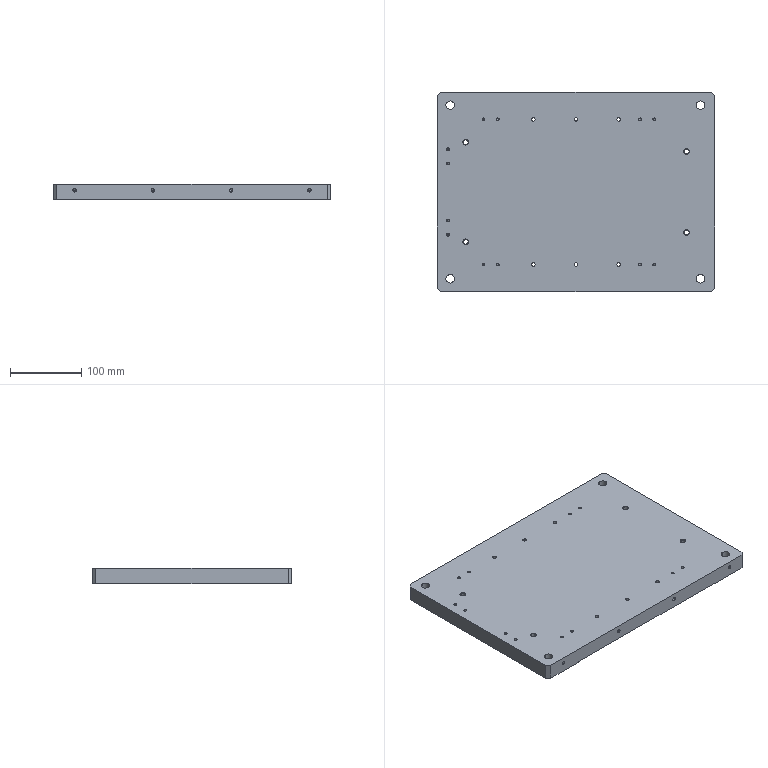NC program | NX | posted with a generic post | part box 390 x 280 x 22 mm
Whole program:
N10 G17 G21 G94 G90
(FLOOR_WALL_COPY , TOOL : D20R0.8)
N12 T01 M6
N14 G54
N16 G17 G0 G90 X208. Y-139.999 S7500 M3
N18 G43 Z30. H1
N20 Z3.
N22 G94 G1 Z0. F1350.
N24 X205.
N26 X-205.
N28 Y-130.262
N30 X205.
N32 Y-120.525
N34 X-205.
N36 Y-115.134
N38 Y-110.788
N40 X205.
N42 Y-101.051
N44 X-205.
N46 Y-91.313
N48 X205.
N50 Y-81.576
N52 X-205.
N54 Y-71.839
N56 X205.
N58 Y-62.102
N60 X-205.
N62 Y-52.365
N64 X205.
N66 Y-42.628
N68 X-205.
N70 Y-32.891
N72 X205.
N74 Y-23.154
N76 X-205.
N78 Y-13.417
N80 X205.
N82 Y-3.68
N84 X-205.
N86 Y6.058
N88 X205.
N90 Y15.795
N92 X-205.
N94 Y25.532
N96 X205.
N98 Y35.269
N100 X-205.
N102 Y45.006
N104 X205.
N106 Y54.743
N108 X-205.
N110 Y64.48
N112 X205.
N114 Y74.217
N116 X-205.
N118 Y83.954
N120 X205.
N122 Y93.692
N124 X-205.
N126 Y103.429
N128 X205.
N130 Y113.166
N132 X-205.
N134 Y122.903
N136 X205.
N138 Y132.64
N140 X-205.
N142 X-208.
N144 Z3.
N146 G0 Z30.
N148 M5
(FLOOR_WALL_1 , TOOL : D10)
N150 T02 M6
N152 G54
N154 G17 G0 G90 X129.897 Y148.1 S9500 M3
N156 G43 Z30. H2
N158 Z2.7
N160 G94 G1 Z-0.3 F2500.
N162 Y145.
N164 Y-145.
N166 X122.474
N168 Y145.
N170 X115.051
N172 Y-145.
N174 X107.629
N176 Y145.
N178 X100.206
N180 Y-145.
N182 X92.783
N184 Y145.
N186 X85.36
N188 Y-145.
N190 X77.938
N192 Y145.
N194 X70.515
N196 Y-145.
N198 X63.092
N200 Y145.
N202 X55.669
N204 Y-145.
N206 X48.247
N208 Y145.
N210 X40.824
N212 Y-145.
N214 X33.401
N216 Y145.
N218 X25.978
N220 Y-145.
N222 X18.555
N224 Y145.
N226 X11.133
N228 Y-145.
N230 X3.71
N232 Y145.
N234 X-3.713
N236 Y-145.
N238 X-11.136
N240 Y145.
N242 X-18.558
N244 Y-145.
N246 X-25.981
N248 Y145.
N250 X-33.404
N252 Y-145.
N254 X-40.827
N256 Y145.
N258 X-48.25
N260 Y-145.
N262 X-55.672
N264 Y145.
N266 X-63.095
N268 Y-145.
N270 X-70.518
N272 Y145.
N274 X-77.941
N276 Y-145.
N278 X-85.363
N280 Y145.
N282 X-92.786
N284 Y-145.
N286 X-100.209
N288 Y145.
N290 X-107.632
N292 Y-145.
N294 X-115.054
N296 Y145.
N298 X-122.477
N300 Y-145.
N302 X-129.9
N304 Y145.
N306 Y148.1
N308 Z2.7
N310 G0 Z30.
N312 X129.897
N314 Z2.4
N316 G1 Z-0.6
N318 Y145.
N320 Y-145.
N322 X122.474
N324 Y145.
N326 X115.051
N328 Y-145.
N330 X107.629
N332 Y145.
N334 X100.206
N336 Y-145.
N338 X92.783
N340 Y145.
N342 X85.36
N344 Y-145.
N346 X77.938
N348 Y145.
N350 X70.515
N352 Y-145.
N354 X63.092
N356 Y145.
N358 X55.669
N360 Y-145.
N362 X48.247
N364 Y145.
N366 X40.824
N368 Y-145.
N370 X33.401
N372 Y145.
N374 X25.978
N376 Y-145.
N378 X18.555
N380 Y145.
N382 X11.133
N384 Y-145.
N386 X3.71
N388 Y145.
N390 X-3.713
N392 Y-145.
N394 X-11.136
N396 Y145.
N398 X-18.558
N400 Y-145.
N402 X-25.981
N404 Y145.
N406 X-33.404
N408 Y-145.
N410 X-40.827
N412 Y145.
N414 X-48.25
N416 Y-145.
N418 X-55.672
N420 Y145.
N422 X-63.095
N424 Y-145.
N426 X-70.518
N428 Y145.
N430 X-77.941
N432 Y-145.
N434 X-85.363
N436 Y145.
N438 X-92.786
N440 Y-145.
N442 X-100.209
N444 Y145.
N446 X-107.632
N448 Y-145.
N450 X-115.054
N452 Y145.
N454 X-122.477
N456 Y-145.
N458 X-129.9
N460 Y145.
N462 Y148.1
N464 Z2.4
N466 G0 Z30.
N468 X129.897
N470 Z2.1
N472 G1 Z-0.9
N474 Y145.
N476 Y-145.
N478 X122.474
N480 Y145.
N482 X115.051
N484 Y-145.
N486 X107.629
N488 Y145.
N490 X100.206
N492 Y-145.
N494 X92.783
N496 Y145.
N498 X85.36
N500 Y-145.
N502 X77.938
N504 Y145.
N506 X70.515
N508 Y-145.
N510 X63.092
N512 Y145.
N514 X55.669
N516 Y-145.
N518 X48.247
N520 Y145.
N522 X40.824
N524 Y-145.
N526 X33.401
N528 Y145.
N530 X25.978
N532 Y-145.
N534 X18.555
N536 Y145.
N538 X11.133
N540 Y-145.
N542 X3.71
N544 Y145.
N546 X-3.713
N548 Y-145.
N550 X-11.136
N552 Y145.
N554 X-18.558
N556 Y-145.
N558 X-25.981
N560 Y145.
N562 X-33.404
N564 Y-145.
N566 X-40.827
N568 Y145.
N570 X-48.25
N572 Y-145.
N574 X-55.672
N576 Y145.
N578 X-63.095
N580 Y-145.
N582 X-70.518
N584 Y145.
N586 X-77.941
N588 Y-145.
N590 X-85.363
N592 Y145.
N594 X-92.786
N596 Y-145.
N598 X-100.209
N600 Y145.
N602 X-107.632
N604 Y-145.
N606 X-115.054
N608 Y145.
N610 X-122.477
N612 Y-145.
N614 X-129.9
N616 Y145.
N618 Y148.1
N620 Z2.1
N622 G0 Z30.
(FLOOR_WALL_1_COPY , TOOL : D10)
N624 X129.999 Y148.
N626 Z2.
N628 G1 Z-1. F1350.
N630 Y145.
N632 Y-145.
N634 X124.999
N636 Y145.
N638 X119.999
N640 Y-145.
N642 X114.999
N644 Y145.
N646 X109.999
N648 Y-145.
N650 X104.999
N652 Y145.
N654 X99.999
N656 Y-145.
N658 X94.999
N660 Y145.
N662 X89.999
N664 Y-145.
N666 X84.999
N668 Y145.
N670 X79.999
N672 Y-145.
N674 X74.999
N676 Y145.
N678 X69.999
N680 Y-145.
N682 X64.999
N684 Y145.
N686 X59.999
N688 Y-145.
N690 X54.999
N692 Y145.
N694 X49.999
N696 Y-145.
N698 X44.999
N700 Y145.
N702 X39.999
N704 Y-145.
N706 X34.999
N708 Y145.
N710 X29.999
N712 Y-145.
N714 X24.999
N716 Y145.
N718 X19.999
N720 Y-145.
N722 X14.999
N724 Y145.
N726 X9.999
N728 Y-145.
N730 X4.999
N732 Y145.
N734 X0.
N736 Y-145.
N738 X-5.
N740 Y145.
N742 X-10.
N744 Y-145.
N746 X-15.
N748 Y145.
N750 X-20.
N752 Y-145.
N754 X-25.
N756 Y145.
N758 X-30.
N760 Y-145.
N762 X-35.
N764 Y145.
N766 X-40.
N768 Y-145.
N770 X-45.
N772 Y145.
N774 X-50.
N776 Y-145.
N778 X-55.
N780 Y145.
N782 X-60.
N784 Y-145.
N786 X-65.
N788 Y145.
N790 X-70.
N792 Y-145.
N794 X-75.
N796 Y145.
N798 X-80.
N800 Y-145.
N802 X-85.
N804 Y145.
N806 X-90.
N808 Y-145.
N810 X-95.
N812 Y145.
N814 X-100.
N816 Y-145.
N818 X-105.
N820 Y145.
N822 X-110.
N824 Y-145.
N826 X-115.
N828 Y145.
N830 X-120.
N832 Y-145.
N834 X-125.
N836 Y145.
N838 X-130.
N840 Y-145.
N842 Y-148.
N844 Z2.
N846 G0 Z30.
N848 M5
(PLANAR_MILL_COPY , TOOL : D6A45)
N850 T07 M6
N852 G54
N854 G17 G0 G90 X-177.866 Y-126.85 S9500 M3
N856 G43 Z30. H7
N858 Z2.25
N860 G94 G1 Z-0.75 F500.
N862 G3 X-177. Y-127.35 R1.
N864 X-171.65 Y-122. R5.35 F1250.
N866 X-177. Y-127.35 R-5.35
N868 X-176.134 Y-126.85 R1.
N870 G1 Z2.25
N872 G0 Z30.
N874 X-133.85 Y0.866
N876 Z2.25
N878 G1 Z-0.75 F500.
N880 G3 X-134.35 Y0. R1.
N882 G1 Y-140. F1250.
N884 G2 X-135. Y-140.65 R0.65
N886 G1 X-190.
N888 G2 X-190.46 Y-140.46 R0.65
N890 G1 X-195.46 Y-135.46
N892 G2 X-195.65 Y-135. R0.65
N894 G1 Y135.
N896 G2 X-195.46 Y135.46 R0.65
N898 G1 X-190.46 Y140.46
N900 G2 X-190. Y140.65 R0.65
N902 G1 X-135.
N904 G2 X-134.35 Y140. R0.65
N906 G1 Y0.
N908 G3 X-133.85 Y-0.866 R1.
N910 G1 Z2.25
N912 G0 Z30.
N914 X-181.85 Y122.866
N916 Z2.25
N918 G1 Z-0.75 F500.
N920 G3 X-182.35 Y122. R1.
N922 X-177. Y116.65 R5.35 F1250.
N924 X-182.35 Y122. R-5.35
N926 X-181.85 Y121.134 R1.
N928 G1 Z2.25
N930 G0 Z30.
N932 X175.866 Y126.85
N934 Z2.25
N936 G1 Z-0.75 F500.
N938 G3 X175. Y127.35 R1.
N940 X169.65 Y122. R5.35 F1250.
N942 X175. Y127.35 R-5.35
N944 X174.134 Y126.85 R1.
N946 G1 Z2.25
N948 G0 Z30.
N950 X133.85 Y-0.866
N952 Z2.25
N954 G1 Z-0.75 F500.
N956 G3 X134.35 Y0. R1.
N958 G1 Y140. F1250.
N960 G2 X135. Y140.65 R0.65
N962 G1 X190.
N964 G2 X190.46 Y140.46 R0.65
N966 G1 X195.46 Y135.46
N968 G2 X195.65 Y135. R0.65
N970 G1 Y-135.
N972 G2 X195.46 Y-135.46 R0.65
N974 G1 X190.46 Y-140.46
N976 G2 X190. Y-140.65 R0.65
N978 G1 X135.
N980 G2 X134.35 Y-140. R0.65
N982 G1 Y0.
N984 G3 X133.85 Y0.866 R1.
N986 G1 Z2.25
N988 G0 Z30.
N990 X174.134 Y-126.85
N992 Z2.25
N994 G1 Z-0.75 F500.
N996 G3 X175. Y-127.35 R1.
N998 X180.35 Y-122. R5.35 F1250.
N1000 X175. Y-127.35 R-5.35
N1002 X175.866 Y-126.85 R1.
N1004 G1 Z2.25
N1006 G0 Z30.
(PLANAR_MILL_COPY_COPY , TOOL : D6A45)
N1008 X132.141 Y-142.349
N1010 Z1.
N1012 G1 Z-2. F500.
N1014 X132.513 Y-141.888
N1016 G3 X132.668 Y-140.9 R1.
N1018 G1 X-132.668 F1250.
N1020 G3 X-132.513 Y-141.888 R1.
N1022 G1 X-132.141 Y-142.349
N1024 Z1.
N1026 G0 Z30.
N1028 Y142.349
N1030 Z1.
N1032 G1 Z-2. F500.
N1034 X-132.513 Y141.888
N1036 G3 X-132.668 Y140.9 R1.
N1038 G1 X132.668 F1250.
N1040 G3 X132.513 Y141.888 R1.
N1042 G1 X132.141 Y142.349
N1044 Z1.
N1046 G0 Z30.
N1048 M5
N1050 M2